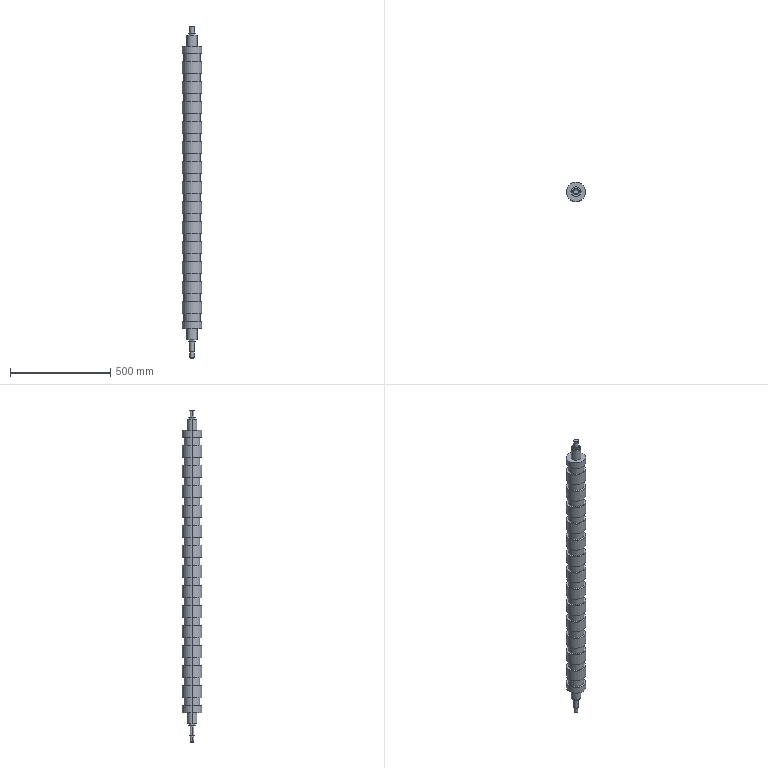Part | SolidWorks | features ICE 6, Chamfer 1, Cut 1, Extrusion 1, LPattern 1, RevCut 1 | 1 solid | 123 faces | box 96 x 96 x 1659 mm | volume 9258344 mm3 | cylinder 72 | plane 37 | cone 14 | commonest cylinder face diameters 96 x30 80 x28 25 x4 32 x4 50 x4 20 x2